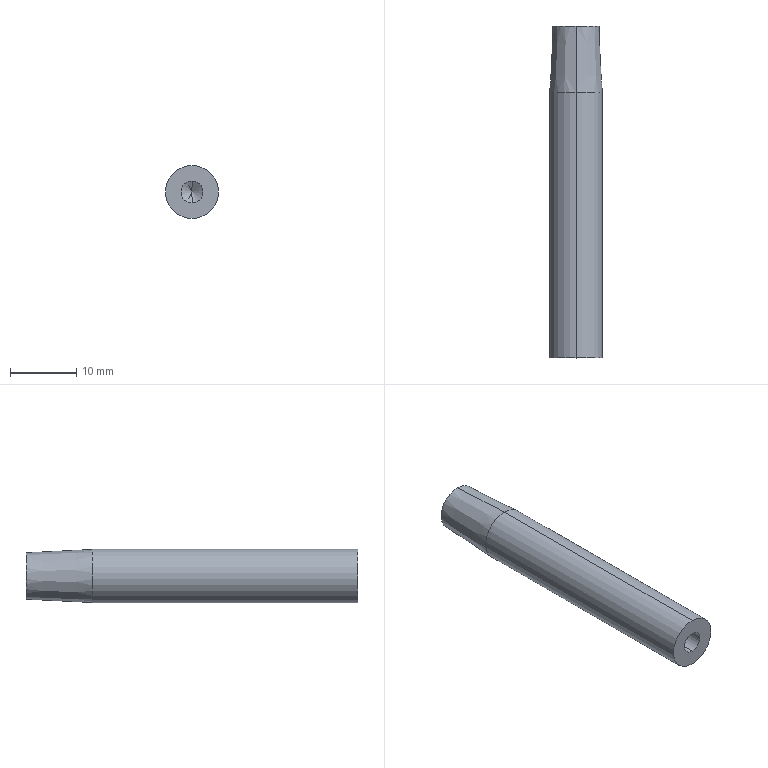Part | SolidWorks | features Chamfer 1, Extrusion 1, HoleWzd 1 | 1 solid | 10 faces | box 8 x 50 x 8 mm | volume 2364 mm3 | cylinder 4 | cone 4 | plane 2 | commonest cylinder face diameters 3.3 x2 8 x2
STEP:
#1=CARTESIAN_POINT('',(0.,10.1,1.65));
#2=VERTEX_POINT('',#1);
#3=CARTESIAN_POINT('',(0.,10.1,-1.65));
#4=VERTEX_POINT('',#3);
#5=CARTESIAN_POINT('',(0.,10.1,0.));
#6=DIRECTION('',(0.,-1.,0.));
#7=DIRECTION('',(0.,0.,-1.));
#8=AXIS2_PLACEMENT_3D('',#5,#6,#7);
#9=CIRCLE('',#8,1.65);
#10=EDGE_CURVE('',#2,#4,#9,.T.);
#11=ORIENTED_EDGE('',*,*,#10,.F.);
#12=CARTESIAN_POINT('',(0.,0.,1.65));
#13=VERTEX_POINT('',#12);
#14=CARTESIAN_POINT('',(0.,0.,1.65));
#15=DIRECTION('',(0.,-1.,0.));
#16=VECTOR('',#15,1000.);
#17=LINE('',#14,#16);
#18=EDGE_CURVE('',#2,#13,#17,.T.);
#19=ORIENTED_EDGE('',*,*,#18,.T.);
#20=CARTESIAN_POINT('',(0.,0.,-1.65));
#21=VERTEX_POINT('',#20);
#22=CARTESIAN_POINT('',(0.,0.,0.));
#23=DIRECTION('',(0.,-1.,0.));
#24=DIRECTION('',(0.,0.,-1.));
#25=AXIS2_PLACEMENT_3D('',#22,#23,#24);
#26=CIRCLE('',#25,1.65);
#27=EDGE_CURVE('',#13,#21,#26,.T.);
#28=ORIENTED_EDGE('',*,*,#27,.T.);
#29=CARTESIAN_POINT('',(0.,0.,-1.65));
#30=DIRECTION('',(0.,-1.,0.));
#31=VECTOR('',#30,1000.);
#32=LINE('',#29,#31);
#33=EDGE_CURVE('',#4,#21,#32,.T.);
#34=ORIENTED_EDGE('',*,*,#33,.F.);
#35=EDGE_LOOP('',(#11,#19,#28,#34));
#36=FACE_OUTER_BOUND('',#35,.T.);
#37=CARTESIAN_POINT('',(0.,0.,0.));
#38=DIRECTION('',(0.,-1.,0.));
#39=DIRECTION('',(0.,0.,-1.));
#40=AXIS2_PLACEMENT_3D('',#37,#38,#39);
#41=CYLINDRICAL_SURFACE('',#40,1.65);
#42=ADVANCED_FACE('',(#36),#41,.F.);
#43=CARTESIAN_POINT('',(0.,11.091,0.));
#44=VERTEX_POINT('',#43);
#45=CARTESIAN_POINT('',(0.,10.1,-1.65));
#46=DIRECTION('',(0.,-0.515,-0.8572));
#47=VECTOR('',#46,1000.);
#48=LINE('',#45,#47);
#49=EDGE_CURVE('',#44,#4,#48,.T.);
#50=ORIENTED_EDGE('',*,*,#49,.F.);
#51=CARTESIAN_POINT('',(0.,10.1,1.65));
#52=DIRECTION('',(0.,-0.515,0.8572));
#53=VECTOR('',#52,1000.);
#54=LINE('',#51,#53);
#55=EDGE_CURVE('',#44,#2,#54,.T.);
#56=ORIENTED_EDGE('',*,*,#55,.T.);
#57=ORIENTED_EDGE('',*,*,#10,.T.);
#58=EDGE_LOOP('',(#50,#56,#57));
#59=FACE_OUTER_BOUND('',#58,.T.);
#60=CARTESIAN_POINT('',(0.,10.1,0.));
#61=DIRECTION('',(0.,-1.,0.));
#62=DIRECTION('',(0.,0.,-1.));
#63=AXIS2_PLACEMENT_3D('',#60,#61,#62);
#64=CONICAL_SURFACE('',#63,1.65,1.03);
#65=ADVANCED_FACE('',(#59),#64,.F.);
#66=CARTESIAN_POINT('',(0.,50.,3.5));
#67=VERTEX_POINT('',#66);
#68=CARTESIAN_POINT('',(0.,50.,-3.5));
#69=VERTEX_POINT('',#68);
#70=CARTESIAN_POINT('',(0.,50.,0.));
#71=DIRECTION('',(0.,1.,0.));
#72=DIRECTION('',(0.,0.,1.));
#73=AXIS2_PLACEMENT_3D('',#70,#71,#72);
#74=CIRCLE('',#73,3.5);
#75=EDGE_CURVE('',#67,#69,#74,.T.);
#76=ORIENTED_EDGE('',*,*,#75,.F.);
#77=CARTESIAN_POINT('',(0.,40.,4.));
#78=VERTEX_POINT('',#77);
#79=CARTESIAN_POINT('',(0.,50.,3.5));
#80=DIRECTION('',(0.,-0.9988,0.04994));
#81=VECTOR('',#80,1000.);
#82=LINE('',#79,#81);
#83=EDGE_CURVE('',#67,#78,#82,.T.);
#84=ORIENTED_EDGE('',*,*,#83,.T.);
#85=CARTESIAN_POINT('',(0.,40.,-4.));
#86=VERTEX_POINT('',#85);
#87=CARTESIAN_POINT('',(0.,40.,0.));
#88=DIRECTION('',(0.,-1.,0.));
#89=DIRECTION('',(0.,0.,1.));
#90=AXIS2_PLACEMENT_3D('',#87,#88,#89);
#91=CIRCLE('',#90,4.);
#92=EDGE_CURVE('',#86,#78,#91,.T.);
#93=ORIENTED_EDGE('',*,*,#92,.F.);
#94=CARTESIAN_POINT('',(0.,50.,-3.5));
#95=DIRECTION('',(0.,-0.9988,-0.04994));
#96=VECTOR('',#95,1000.);
#97=LINE('',#94,#96);
#98=EDGE_CURVE('',#69,#86,#97,.T.);
#99=ORIENTED_EDGE('',*,*,#98,.F.);
#100=EDGE_LOOP('',(#76,#84,#93,#99));
#101=FACE_OUTER_BOUND('',#100,.T.);
#102=CARTESIAN_POINT('',(0.,50.,0.));
#103=DIRECTION('',(0.,-1.,0.));
#104=DIRECTION('',(0.,0.,-1.));
#105=AXIS2_PLACEMENT_3D('',#102,#103,#104);
#106=CONICAL_SURFACE('',#105,3.5,0.04996);
#107=ADVANCED_FACE('',(#101),#106,.T.);
#108=ORIENTED_EDGE('',*,*,#92,.T.);
#109=CARTESIAN_POINT('',(0.,0.,4.));
#110=VERTEX_POINT('',#109);
#111=CARTESIAN_POINT('',(0.,50.,4.));
#112=DIRECTION('',(0.,-1.,0.));
#113=VECTOR('',#112,1000.);
#114=LINE('',#111,#113);
#115=EDGE_CURVE('',#78,#110,#114,.T.);
#116=ORIENTED_EDGE('',*,*,#115,.T.);
#117=CARTESIAN_POINT('',(0.,0.,-4.));
#118=VERTEX_POINT('',#117);
#119=CARTESIAN_POINT('',(0.,0.,0.));
#120=DIRECTION('',(0.,1.,0.));
#121=DIRECTION('',(0.,0.,1.));
#122=AXIS2_PLACEMENT_3D('',#119,#120,#121);
#123=CIRCLE('',#122,4.);
#124=EDGE_CURVE('',#110,#118,#123,.T.);
#125=ORIENTED_EDGE('',*,*,#124,.T.);
#126=CARTESIAN_POINT('',(0.,50.,-4.));
#127=DIRECTION('',(0.,-1.,0.));
#128=VECTOR('',#127,1000.);
#129=LINE('',#126,#128);
#130=EDGE_CURVE('',#86,#118,#129,.T.);
#131=ORIENTED_EDGE('',*,*,#130,.F.);
#132=EDGE_LOOP('',(#108,#116,#125,#131));
#133=FACE_OUTER_BOUND('',#132,.T.);
#134=CARTESIAN_POINT('',(0.,50.,0.));
#135=DIRECTION('',(0.,-1.,0.));
#136=DIRECTION('',(0.,0.,-1.));
#137=AXIS2_PLACEMENT_3D('',#134,#135,#136);
#138=CYLINDRICAL_SURFACE('',#137,4.);
#139=ADVANCED_FACE('',(#133),#138,.T.);
#140=ORIENTED_EDGE('',*,*,#115,.F.);
#141=CARTESIAN_POINT('',(0.,40.,0.));
#142=DIRECTION('',(0.,-1.,0.));
#143=DIRECTION('',(0.,0.,1.));
#144=AXIS2_PLACEMENT_3D('',#141,#142,#143);
#145=CIRCLE('',#144,4.);
#146=EDGE_CURVE('',#78,#86,#145,.T.);
#147=ORIENTED_EDGE('',*,*,#146,.T.);
#148=ORIENTED_EDGE('',*,*,#130,.T.);
#149=CARTESIAN_POINT('',(0.,0.,0.));
#150=DIRECTION('',(0.,1.,0.));
#151=DIRECTION('',(0.,0.,1.));
#152=AXIS2_PLACEMENT_3D('',#149,#150,#151);
#153=CIRCLE('',#152,4.);
#154=EDGE_CURVE('',#118,#110,#153,.T.);
#155=ORIENTED_EDGE('',*,*,#154,.T.);
#156=EDGE_LOOP('',(#140,#147,#148,#155));
#157=FACE_OUTER_BOUND('',#156,.T.);
#158=CARTESIAN_POINT('',(0.,50.,0.));
#159=DIRECTION('',(0.,-1.,0.));
#160=DIRECTION('',(0.,0.,-1.));
#161=AXIS2_PLACEMENT_3D('',#158,#159,#160);
#162=CYLINDRICAL_SURFACE('',#161,4.);
#163=ADVANCED_FACE('',(#157),#162,.T.);
#164=CARTESIAN_POINT('',(0.,50.,0.));
#165=DIRECTION('',(0.,1.,0.));
#166=DIRECTION('',(0.,0.,1.));
#167=AXIS2_PLACEMENT_3D('',#164,#165,#166);
#168=CIRCLE('',#167,3.5);
#169=EDGE_CURVE('',#69,#67,#168,.T.);
#170=ORIENTED_EDGE('',*,*,#169,.T.);
#171=ORIENTED_EDGE('',*,*,#75,.T.);
#172=EDGE_LOOP('',(#170,#171));
#173=FACE_OUTER_BOUND('',#172,.T.);
#174=CARTESIAN_POINT('',(0.,50.,0.));
#175=DIRECTION('',(0.,1.,0.));
#176=DIRECTION('',(0.,0.,1.));
#177=AXIS2_PLACEMENT_3D('',#174,#175,#176);
#178=PLANE('',#177);
#179=ADVANCED_FACE('',(#173),#178,.T.);
#180=CARTESIAN_POINT('',(0.,0.,0.));
#181=DIRECTION('',(0.,-1.,0.));
#182=DIRECTION('',(0.,0.,-1.));
#183=AXIS2_PLACEMENT_3D('',#180,#181,#182);
#184=CIRCLE('',#183,1.65);
#185=EDGE_CURVE('',#21,#13,#184,.T.);
#186=ORIENTED_EDGE('',*,*,#185,.F.);
#187=ORIENTED_EDGE('',*,*,#27,.F.);
#188=EDGE_LOOP('',(#186,#187));
#189=FACE_BOUND('',#188,.T.);
#190=ORIENTED_EDGE('',*,*,#154,.F.);
#191=ORIENTED_EDGE('',*,*,#124,.F.);
#192=EDGE_LOOP('',(#190,#191));
#193=FACE_OUTER_BOUND('',#192,.T.);
#194=CARTESIAN_POINT('',(0.,0.,0.));
#195=DIRECTION('',(0.,1.,0.));
#196=DIRECTION('',(0.,0.,1.));
#197=AXIS2_PLACEMENT_3D('',#194,#195,#196);
#198=PLANE('',#197);
#199=ADVANCED_FACE('',(#189,#193),#198,.F.);
#200=ORIENTED_EDGE('',*,*,#83,.F.);
#201=ORIENTED_EDGE('',*,*,#169,.F.);
#202=ORIENTED_EDGE('',*,*,#98,.T.);
#203=ORIENTED_EDGE('',*,*,#146,.F.);
#204=EDGE_LOOP('',(#200,#201,#202,#203));
#205=FACE_OUTER_BOUND('',#204,.T.);
#206=CARTESIAN_POINT('',(0.,50.,0.));
#207=DIRECTION('',(0.,-1.,0.));
#208=DIRECTION('',(0.,0.,-1.));
#209=AXIS2_PLACEMENT_3D('',#206,#207,#208);
#210=CONICAL_SURFACE('',#209,3.5,0.04996);
#211=ADVANCED_FACE('',(#205),#210,.T.);
#212=ORIENTED_EDGE('',*,*,#55,.F.);
#213=ORIENTED_EDGE('',*,*,#49,.T.);
#214=CARTESIAN_POINT('',(0.,10.1,0.));
#215=DIRECTION('',(0.,-1.,0.));
#216=DIRECTION('',(0.,0.,-1.));
#217=AXIS2_PLACEMENT_3D('',#214,#215,#216);
#218=CIRCLE('',#217,1.65);
#219=EDGE_CURVE('',#4,#2,#218,.T.);
#220=ORIENTED_EDGE('',*,*,#219,.T.);
#221=EDGE_LOOP('',(#212,#213,#220));
#222=FACE_OUTER_BOUND('',#221,.T.);
#223=CARTESIAN_POINT('',(0.,10.1,0.));
#224=DIRECTION('',(0.,-1.,0.));
#225=DIRECTION('',(0.,0.,-1.));
#226=AXIS2_PLACEMENT_3D('',#223,#224,#225);
#227=CONICAL_SURFACE('',#226,1.65,1.03);
#228=ADVANCED_FACE('',(#222),#227,.F.);
#229=ORIENTED_EDGE('',*,*,#18,.F.);
#230=ORIENTED_EDGE('',*,*,#219,.F.);
#231=ORIENTED_EDGE('',*,*,#33,.T.);
#232=ORIENTED_EDGE('',*,*,#185,.T.);
#233=EDGE_LOOP('',(#229,#230,#231,#232));
#234=FACE_OUTER_BOUND('',#233,.T.);
#235=CARTESIAN_POINT('',(0.,0.,0.));
#236=DIRECTION('',(0.,-1.,0.));
#237=DIRECTION('',(0.,0.,-1.));
#238=AXIS2_PLACEMENT_3D('',#235,#236,#237);
#239=CYLINDRICAL_SURFACE('',#238,1.65);
#240=ADVANCED_FACE('',(#234),#239,.F.);
#241=CLOSED_SHELL('',(#42,#65,#107,#139,#163,#179,#199,#211,#228,#240));
#242=MANIFOLD_SOLID_BREP('',#241);
#243=CARTESIAN_POINT('',(0.,0.,0.));
#244=DIRECTION('',(0.,0.,1.));
#245=DIRECTION('',(1.,0.,0.));
#246=AXIS2_PLACEMENT_3D('',#243,#244,#245);
#247=(LENGTH_UNIT()NAMED_UNIT(*)SI_UNIT(.MILLI.,.METRE.));
#248=UNCERTAINTY_MEASURE_WITH_UNIT(LENGTH_MEASURE(0.00001),#247,'','');
#249=(NAMED_UNIT(*)PLANE_ANGLE_UNIT()SI_UNIT($,.RADIAN.));
#250=(NAMED_UNIT(*)SI_UNIT($,.STERADIAN.)SOLID_ANGLE_UNIT());
#251=(GEOMETRIC_REPRESENTATION_CONTEXT(3)GLOBAL_UNCERTAINTY_ASSIGNED_CONTEXT((#248))GLOBAL_UNIT_ASSIGNED_CONTEXT((#247,#249,#250))REPRESENTATION_CONTEXT('',''));
#252=ADVANCED_BREP_SHAPE_REPRESENTATION('',(#242,#246),#251);